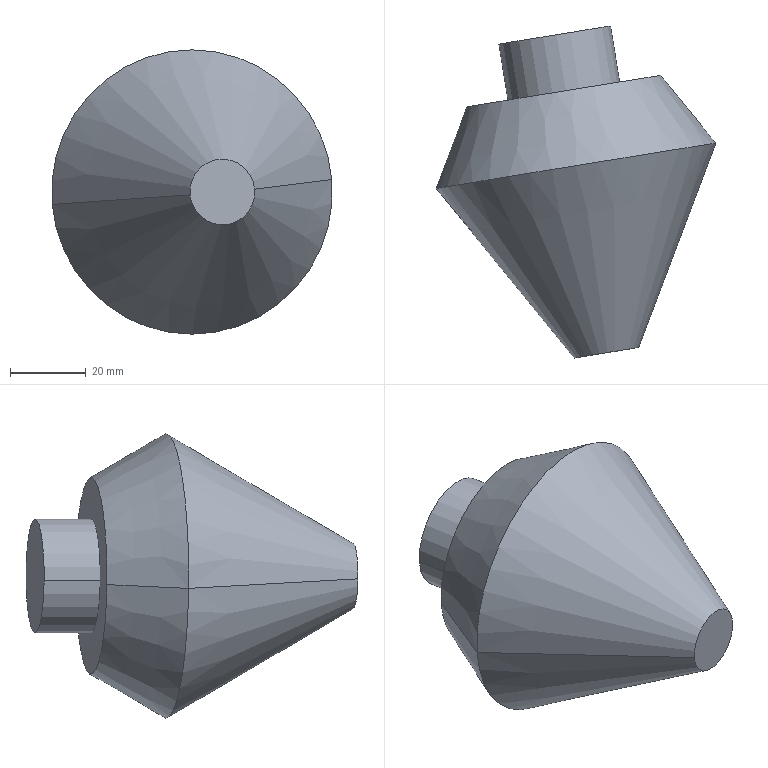Part | SolidWorks | features SplitBody 1 | 1 solid | 9 faces | box 74.124 x 87.696 x 75.094 mm | volume 169557 mm3 | cone 4 | plane 3 | cylinder 2 | commonest cylinder face diameters 30 x2
STEP:
#1=CARTESIAN_POINT('',(4117.079,-1.55,-818.256));
#2=VERTEX_POINT('',#1);
#3=CARTESIAN_POINT('',(4134.149,1.22,-816.744));
#4=VERTEX_POINT('',#3);
#5=CARTESIAN_POINT('',(4125.614,-0.1648,-817.5));
#6=DIRECTION('',(-0.1602,0.9871,0.));
#7=DIRECTION('',(-0.9833,-0.1596,-0.08716));
#8=AXIS2_PLACEMENT_3D('',#5,#6,#7);
#9=CIRCLE('',#8,8.679);
#10=EDGE_CURVE('',#2,#4,#9,.T.);
#11=ORIENTED_EDGE('',*,*,#10,.T.);
#12=CARTESIAN_POINT('',(4154.525,55.181,-814.228));
#13=VERTEX_POINT('',#12);
#14=CARTESIAN_POINT('',(4154.525,55.181,-814.228));
#15=DIRECTION('',(0.3529,0.9346,0.04358));
#16=VECTOR('',#15,1000.);
#17=LINE('',#14,#16);
#18=EDGE_CURVE('',#4,#13,#17,.T.);
#19=ORIENTED_EDGE('',*,*,#18,.T.);
#20=CARTESIAN_POINT('',(4080.683,43.197,-820.772));
#21=VERTEX_POINT('',#20);
#22=CARTESIAN_POINT('',(4117.604,49.189,-817.5));
#23=DIRECTION('',(0.1602,-0.9871,0.));
#24=DIRECTION('',(-0.9833,-0.1596,-0.08716));
#25=AXIS2_PLACEMENT_3D('',#22,#23,#24);
#26=CIRCLE('',#25,37.547);
#27=EDGE_CURVE('',#13,#21,#26,.T.);
#28=ORIENTED_EDGE('',*,*,#27,.T.);
#29=CARTESIAN_POINT('',(4080.683,43.197,-820.772));
#30=DIRECTION('',(-0.6304,0.775,-0.04358));
#31=VECTOR('',#30,1000.);
#32=LINE('',#29,#31);
#33=EDGE_CURVE('',#2,#21,#32,.T.);
#34=ORIENTED_EDGE('',*,*,#33,.F.);
#35=EDGE_LOOP('',(#11,#19,#28,#34));
#36=FACE_OUTER_BOUND('',#35,.T.);
#37=CARTESIAN_POINT('',(4117.604,49.189,-817.5));
#38=DIRECTION('',(-0.1602,0.9871,0.));
#39=DIRECTION('',(-0.9833,-0.1596,-0.08716));
#40=AXIS2_PLACEMENT_3D('',#37,#38,#39);
#41=CONICAL_SURFACE('',#40,37.547,0.5236);
#42=ADVANCED_FACE('',(#36),#41,.T.);
#43=CARTESIAN_POINT('',(4139.967,73.08,-815.234));
#44=VERTEX_POINT('',#43);
#45=CARTESIAN_POINT('',(4088.833,64.782,-819.766));
#46=VERTEX_POINT('',#45);
#47=CARTESIAN_POINT('',(4114.4,68.931,-817.5));
#48=DIRECTION('',(0.1602,-0.9871,0.));
#49=DIRECTION('',(0.9833,0.1596,0.08716));
#50=AXIS2_PLACEMENT_3D('',#47,#48,#49);
#51=CIRCLE('',#50,26.);
#52=EDGE_CURVE('',#44,#46,#51,.T.);
#53=ORIENTED_EDGE('',*,*,#52,.T.);
#54=CARTESIAN_POINT('',(4080.683,43.197,-820.772));
#55=DIRECTION('',(-0.3529,-0.9346,-0.04358));
#56=VECTOR('',#55,1000.);
#57=LINE('',#54,#56);
#58=EDGE_CURVE('',#46,#21,#57,.T.);
#59=ORIENTED_EDGE('',*,*,#58,.T.);
#60=ORIENTED_EDGE('',*,*,#27,.F.);
#61=CARTESIAN_POINT('',(4154.525,55.181,-814.228));
#62=DIRECTION('',(0.6304,-0.775,0.04358));
#63=VECTOR('',#62,1000.);
#64=LINE('',#61,#63);
#65=EDGE_CURVE('',#44,#13,#64,.T.);
#66=ORIENTED_EDGE('',*,*,#65,.F.);
#67=EDGE_LOOP('',(#53,#59,#60,#66));
#68=FACE_OUTER_BOUND('',#67,.T.);
#69=CARTESIAN_POINT('',(4117.604,49.189,-817.5));
#70=DIRECTION('',(0.1602,-0.9871,0.));
#71=DIRECTION('',(0.9833,0.1596,0.08716));
#72=AXIS2_PLACEMENT_3D('',#69,#70,#71);
#73=CONICAL_SURFACE('',#72,37.547,0.5236);
#74=ADVANCED_FACE('',(#68),#73,.T.);
#75=CARTESIAN_POINT('',(4129.15,71.325,-816.193));
#76=VERTEX_POINT('',#75);
#77=CARTESIAN_POINT('',(4099.65,66.537,-818.807));
#78=VERTEX_POINT('',#77);
#79=CARTESIAN_POINT('',(4114.4,68.931,-817.5));
#80=DIRECTION('',(0.1602,-0.9871,0.));
#81=DIRECTION('',(-0.9833,-0.1596,-0.08716));
#82=AXIS2_PLACEMENT_3D('',#79,#80,#81);
#83=CIRCLE('',#82,15.);
#84=EDGE_CURVE('',#76,#78,#83,.T.);
#85=ORIENTED_EDGE('',*,*,#84,.F.);
#86=CARTESIAN_POINT('',(4126.747,86.131,-816.193));
#87=VERTEX_POINT('',#86);
#88=CARTESIAN_POINT('',(4126.747,86.131,-816.193));
#89=DIRECTION('',(-0.1602,0.9871,0.));
#90=VECTOR('',#89,1000.);
#91=LINE('',#88,#90);
#92=EDGE_CURVE('',#76,#87,#91,.T.);
#93=ORIENTED_EDGE('',*,*,#92,.T.);
#94=CARTESIAN_POINT('',(4097.247,81.344,-818.807));
#95=VERTEX_POINT('',#94);
#96=CARTESIAN_POINT('',(4111.997,83.737,-817.5));
#97=DIRECTION('',(0.1602,-0.9871,0.));
#98=DIRECTION('',(-0.9833,-0.1596,-0.08716));
#99=AXIS2_PLACEMENT_3D('',#96,#97,#98);
#100=CIRCLE('',#99,15.);
#101=EDGE_CURVE('',#87,#95,#100,.T.);
#102=ORIENTED_EDGE('',*,*,#101,.T.);
#103=CARTESIAN_POINT('',(4097.247,81.344,-818.807));
#104=DIRECTION('',(-0.1602,0.9871,0.));
#105=VECTOR('',#104,1000.);
#106=LINE('',#103,#105);
#107=EDGE_CURVE('',#78,#95,#106,.T.);
#108=ORIENTED_EDGE('',*,*,#107,.F.);
#109=EDGE_LOOP('',(#85,#93,#102,#108));
#110=FACE_OUTER_BOUND('',#109,.T.);
#111=CARTESIAN_POINT('',(4111.997,83.737,-817.5));
#112=DIRECTION('',(-0.1602,0.9871,0.));
#113=DIRECTION('',(-0.9833,-0.1596,-0.08716));
#114=AXIS2_PLACEMENT_3D('',#111,#112,#113);
#115=CYLINDRICAL_SURFACE('',#114,15.);
#116=ADVANCED_FACE('',(#110),#115,.T.);
#117=ORIENTED_EDGE('',*,*,#18,.F.);
#118=CARTESIAN_POINT('',(4125.614,-0.1648,-817.5));
#119=DIRECTION('',(-0.1602,0.9871,0.));
#120=DIRECTION('',(-0.9833,-0.1596,-0.08716));
#121=AXIS2_PLACEMENT_3D('',#118,#119,#120);
#122=CIRCLE('',#121,8.679);
#123=EDGE_CURVE('',#4,#2,#122,.T.);
#124=ORIENTED_EDGE('',*,*,#123,.T.);
#125=ORIENTED_EDGE('',*,*,#33,.T.);
#126=CARTESIAN_POINT('',(4117.604,49.189,-817.5));
#127=DIRECTION('',(0.1602,-0.9871,0.));
#128=DIRECTION('',(-0.9833,-0.1596,-0.08716));
#129=AXIS2_PLACEMENT_3D('',#126,#127,#128);
#130=CIRCLE('',#129,37.547);
#131=EDGE_CURVE('',#21,#13,#130,.T.);
#132=ORIENTED_EDGE('',*,*,#131,.T.);
#133=EDGE_LOOP('',(#117,#124,#125,#132));
#134=FACE_OUTER_BOUND('',#133,.T.);
#135=CARTESIAN_POINT('',(4117.604,49.189,-817.5));
#136=DIRECTION('',(-0.1602,0.9871,0.));
#137=DIRECTION('',(-0.9833,-0.1596,-0.08716));
#138=AXIS2_PLACEMENT_3D('',#135,#136,#137);
#139=CONICAL_SURFACE('',#138,37.547,0.5236);
#140=ADVANCED_FACE('',(#134),#139,.T.);
#141=ORIENTED_EDGE('',*,*,#58,.F.);
#142=CARTESIAN_POINT('',(4114.4,68.931,-817.5));
#143=DIRECTION('',(0.1602,-0.9871,0.));
#144=DIRECTION('',(0.9833,0.1596,0.08716));
#145=AXIS2_PLACEMENT_3D('',#142,#143,#144);
#146=CIRCLE('',#145,26.);
#147=EDGE_CURVE('',#46,#44,#146,.T.);
#148=ORIENTED_EDGE('',*,*,#147,.T.);
#149=ORIENTED_EDGE('',*,*,#65,.T.);
#150=ORIENTED_EDGE('',*,*,#131,.F.);
#151=EDGE_LOOP('',(#141,#148,#149,#150));
#152=FACE_OUTER_BOUND('',#151,.T.);
#153=CARTESIAN_POINT('',(4117.604,49.189,-817.5));
#154=DIRECTION('',(0.1602,-0.9871,0.));
#155=DIRECTION('',(0.9833,0.1596,0.08716));
#156=AXIS2_PLACEMENT_3D('',#153,#154,#155);
#157=CONICAL_SURFACE('',#156,37.547,0.5236);
#158=ADVANCED_FACE('',(#152),#157,.T.);
#159=ORIENTED_EDGE('',*,*,#10,.F.);
#160=ORIENTED_EDGE('',*,*,#123,.F.);
#161=EDGE_LOOP('',(#159,#160));
#162=FACE_OUTER_BOUND('',#161,.T.);
#163=CARTESIAN_POINT('',(4144.074,2.831,-815.864));
#164=DIRECTION('',(0.1602,-0.9871,0.));
#165=DIRECTION('',(0.9833,0.1596,0.08716));
#166=AXIS2_PLACEMENT_3D('',#163,#164,#165);
#167=PLANE('',#166);
#168=ADVANCED_FACE('',(#162),#167,.T.);
#169=CARTESIAN_POINT('',(4114.4,68.931,-817.5));
#170=DIRECTION('',(0.1602,-0.9871,0.));
#171=DIRECTION('',(-0.9833,-0.1596,-0.08716));
#172=AXIS2_PLACEMENT_3D('',#169,#170,#171);
#173=CIRCLE('',#172,15.);
#174=EDGE_CURVE('',#78,#76,#173,.T.);
#175=ORIENTED_EDGE('',*,*,#174,.T.);
#176=ORIENTED_EDGE('',*,*,#84,.T.);
#177=EDGE_LOOP('',(#175,#176));
#178=FACE_BOUND('',#177,.T.);
#179=ORIENTED_EDGE('',*,*,#52,.F.);
#180=ORIENTED_EDGE('',*,*,#147,.F.);
#181=EDGE_LOOP('',(#179,#180));
#182=FACE_OUTER_BOUND('',#181,.T.);
#183=CARTESIAN_POINT('',(4132.861,71.927,-815.864));
#184=DIRECTION('',(-0.1602,0.9871,0.));
#185=DIRECTION('',(-0.9833,-0.1596,-0.08716));
#186=AXIS2_PLACEMENT_3D('',#183,#184,#185);
#187=PLANE('',#186);
#188=ADVANCED_FACE('',(#178,#182),#187,.T.);
#189=ORIENTED_EDGE('',*,*,#92,.F.);
#190=ORIENTED_EDGE('',*,*,#174,.F.);
#191=ORIENTED_EDGE('',*,*,#107,.T.);
#192=CARTESIAN_POINT('',(4111.997,83.737,-817.5));
#193=DIRECTION('',(0.1602,-0.9871,0.));
#194=DIRECTION('',(-0.9833,-0.1596,-0.08716));
#195=AXIS2_PLACEMENT_3D('',#192,#193,#194);
#196=CIRCLE('',#195,15.);
#197=EDGE_CURVE('',#95,#87,#196,.T.);
#198=ORIENTED_EDGE('',*,*,#197,.T.);
#199=EDGE_LOOP('',(#189,#190,#191,#198));
#200=FACE_OUTER_BOUND('',#199,.T.);
#201=CARTESIAN_POINT('',(4111.997,83.737,-817.5));
#202=DIRECTION('',(-0.1602,0.9871,0.));
#203=DIRECTION('',(-0.9833,-0.1596,-0.08716));
#204=AXIS2_PLACEMENT_3D('',#201,#202,#203);
#205=CYLINDRICAL_SURFACE('',#204,15.);
#206=ADVANCED_FACE('',(#200),#205,.T.);
#207=ORIENTED_EDGE('',*,*,#197,.F.);
#208=ORIENTED_EDGE('',*,*,#101,.F.);
#209=EDGE_LOOP('',(#207,#208));
#210=FACE_OUTER_BOUND('',#209,.T.);
#211=CARTESIAN_POINT('',(4130.458,86.733,-815.864));
#212=DIRECTION('',(-0.1602,0.9871,0.));
#213=DIRECTION('',(-0.9833,-0.1596,-0.08716));
#214=AXIS2_PLACEMENT_3D('',#211,#212,#213);
#215=PLANE('',#214);
#216=ADVANCED_FACE('',(#210),#215,.T.);
#217=CLOSED_SHELL('',(#42,#74,#116,#140,#158,#168,#188,#206,#216));
#218=MANIFOLD_SOLID_BREP('',#217);
#219=CARTESIAN_POINT('',(0.,0.,0.));
#220=DIRECTION('',(0.,0.,1.));
#221=DIRECTION('',(1.,0.,0.));
#222=AXIS2_PLACEMENT_3D('',#219,#220,#221);
#223=(LENGTH_UNIT()NAMED_UNIT(*)SI_UNIT(.MILLI.,.METRE.));
#224=UNCERTAINTY_MEASURE_WITH_UNIT(LENGTH_MEASURE(0.00001),#223,'','');
#225=(NAMED_UNIT(*)PLANE_ANGLE_UNIT()SI_UNIT($,.RADIAN.));
#226=(NAMED_UNIT(*)SI_UNIT($,.STERADIAN.)SOLID_ANGLE_UNIT());
#227=(GEOMETRIC_REPRESENTATION_CONTEXT(3)GLOBAL_UNCERTAINTY_ASSIGNED_CONTEXT((#224))GLOBAL_UNIT_ASSIGNED_CONTEXT((#223,#225,#226))REPRESENTATION_CONTEXT('',''));
#228=ADVANCED_BREP_SHAPE_REPRESENTATION('',(#218,#222),#227);